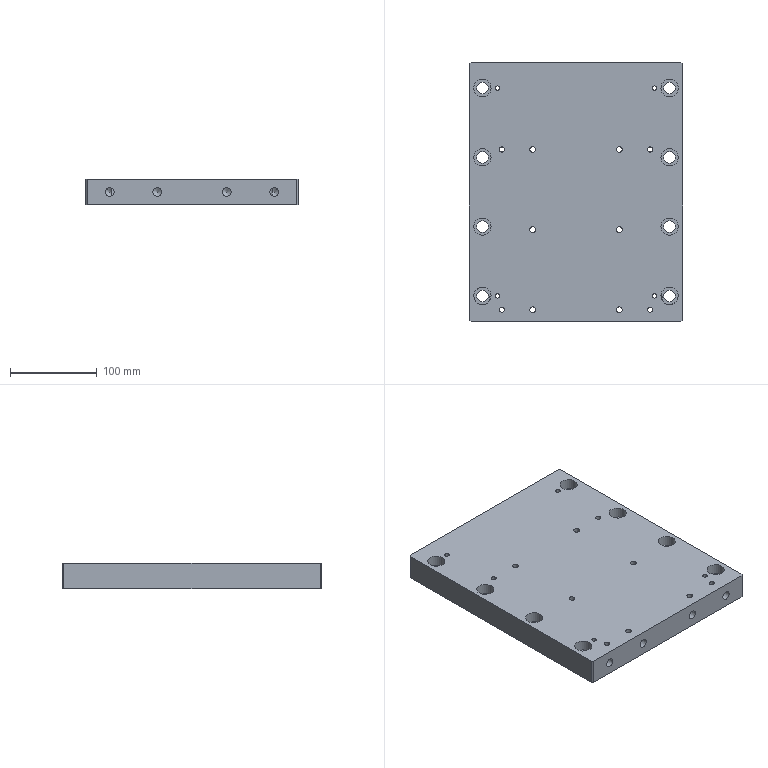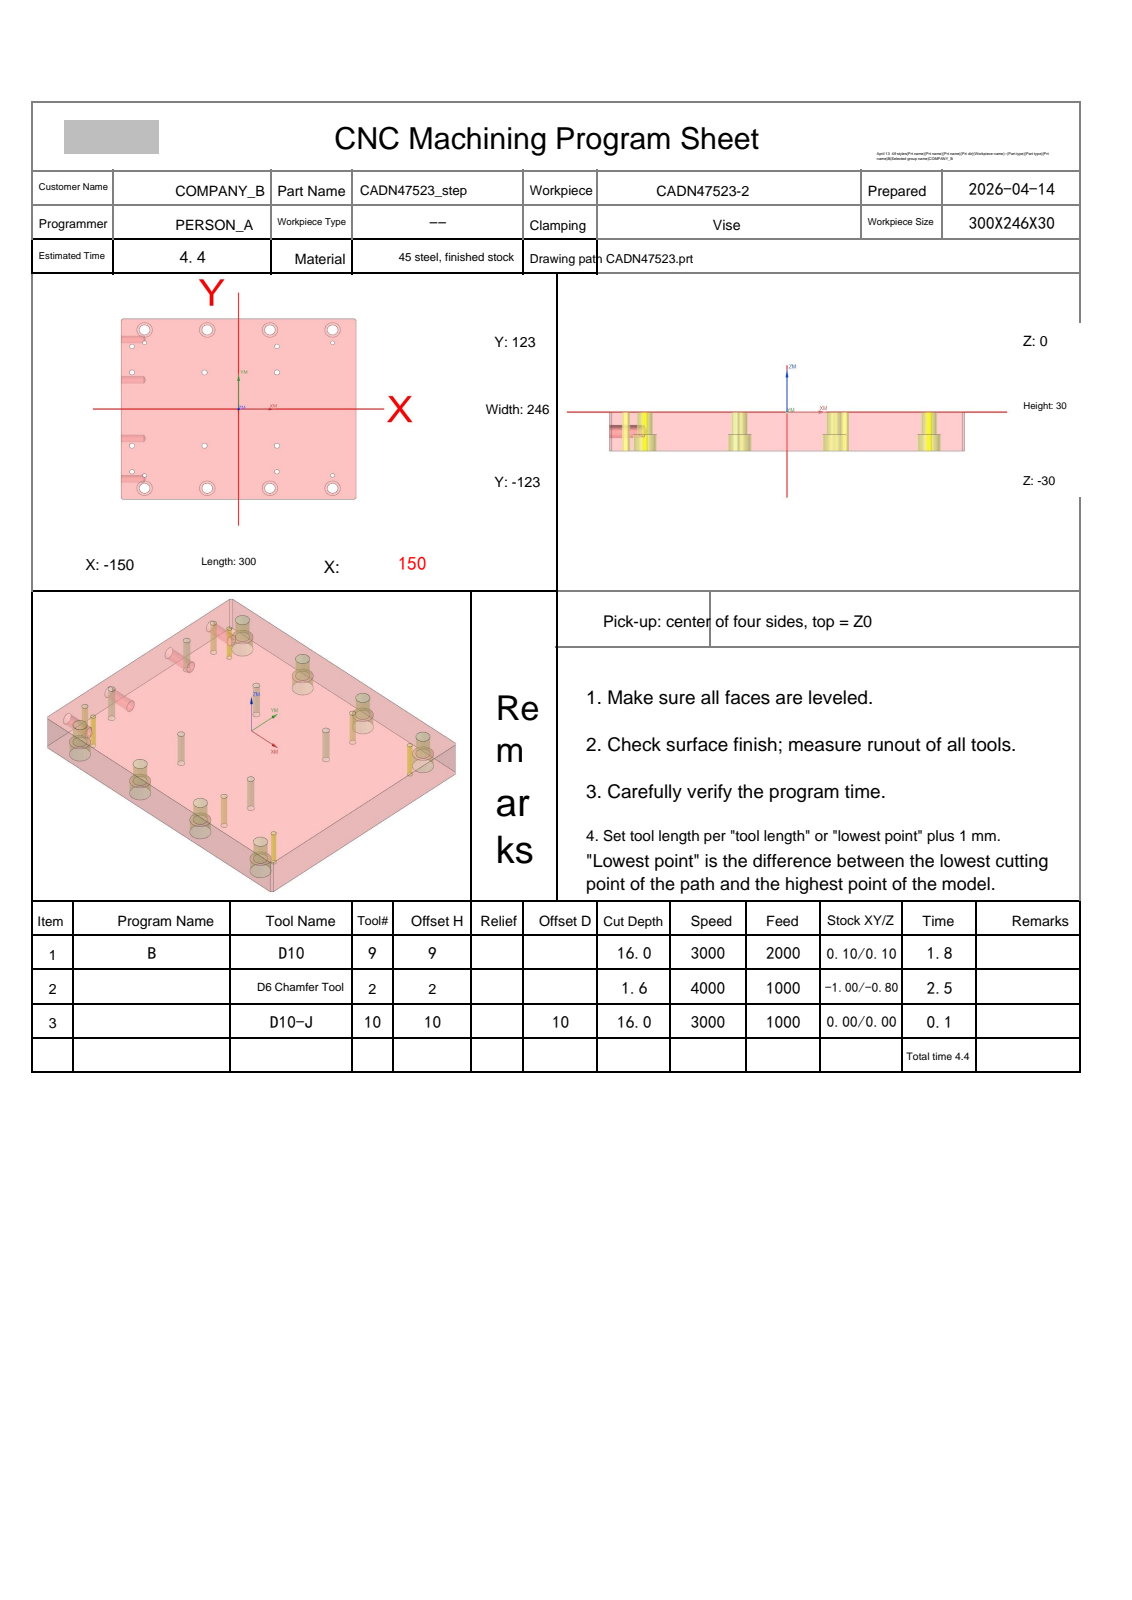NC program | NX | posted by the shop | part box 246 x 300 x 30 mm
Whole program:
%
O0001
(Machine time: 4.96 MIN)
(===Total Tool:3===)
(T9=D10     D=10.  R=0.   D-  H09 Z=-16.  )
(T2=D6 Chamfer Tool   D=6.   R=0.   D-  H02 Z=-1.6  )
(T10=D10-J  D=10.  R=0.   D10 H10 Z=-16.  )
G80 G90 G17 G49 G40
G91 G28 Z0
M01
N1 T09 M06
(D10  D=10. R=0. H=09 ce=0.10 di=0.10)
G00 G90 G54 X160.1 Y-118.112 M03 S3000
G43 H09 Z20.
M08
Z-.4
G01 X153.606 Y-124.606 F2000.
X151.606 Y-126.606
X145.112 Y-133.1
G00 Z-.8
G01 X151.606 Y-126.606
X153.606 Y-124.606
X160.1 Y-118.112
G00 Z-1.2
G01 X153.606 Y-124.606
X151.606 Y-126.606
X145.112 Y-133.1
G00 Z-1.6
G01 X151.606 Y-126.606
X153.606 Y-124.606
X160.1 Y-118.112
G00 Z-2.
G01 X153.606 Y-124.606
X151.606 Y-126.606
X145.112 Y-133.1
G00 Z-2.4
G01 X151.606 Y-126.606
X153.606 Y-124.606
X160.1 Y-118.112
G00 Z-2.8
G01 X153.606 Y-124.606
X151.606 Y-126.606
X145.112 Y-133.1
G00 Z-3.2
G01 X151.606 Y-126.606
X153.606 Y-124.606
X160.1 Y-118.112
G00 Z-3.6
G01 X153.606 Y-124.606
X151.606 Y-126.606
X145.112 Y-133.1
G00 Z-4.
G01 X151.606 Y-126.606
X153.606 Y-124.606
X160.1 Y-118.112
G00 Z-4.4
G01 X153.606 Y-124.606
X151.606 Y-126.606
X145.112 Y-133.1
G00 Z-4.8
G01 X151.606 Y-126.606
X153.606 Y-124.606
X160.1 Y-118.112
G00 Z-5.2
G01 X153.606 Y-124.606
X151.606 Y-126.606
X145.112 Y-133.1
G00 Z-5.6
G01 X151.606 Y-126.606
X153.606 Y-124.606
X160.1 Y-118.112
G00 Z-6.
G01 X153.606 Y-124.606
X151.606 Y-126.606
X145.112 Y-133.1
G00 Z-6.4
G01 X151.606 Y-126.606
X153.606 Y-124.606
X160.1 Y-118.112
G00 Z-6.8
G01 X153.606 Y-124.606
X151.606 Y-126.606
X145.112 Y-133.1
G00 Z-7.2
G01 X151.606 Y-126.606
X153.606 Y-124.606
X160.1 Y-118.112
G00 Z-7.6
G01 X153.606 Y-124.606
X151.606 Y-126.606
X145.112 Y-133.1
G00 Z-8.
G01 X151.606 Y-126.606
X153.606 Y-124.606
X160.1 Y-118.112
G00 Z-8.4
G01 X153.606 Y-124.606
X151.606 Y-126.606
X145.112 Y-133.1
G00 Z-8.8
G01 X151.606 Y-126.606
X153.606 Y-124.606
X160.1 Y-118.112
G00 Z-9.2
G01 X153.606 Y-124.606
X151.606 Y-126.606
X145.112 Y-133.1
G00 Z-9.6
G01 X151.606 Y-126.606
X153.606 Y-124.606
X160.1 Y-118.112
G00 Z-10.
G01 X153.606 Y-124.606
X151.606 Y-126.606
X145.112 Y-133.1
G00 Z-10.4
G01 X151.606 Y-126.606
X153.606 Y-124.606
X160.1 Y-118.112
G00 Z-10.8
G01 X153.606 Y-124.606
X151.606 Y-126.606
X145.112 Y-133.1
G00 Z-11.2
G01 X151.606 Y-126.606
X153.606 Y-124.606
X160.1 Y-118.112
G00 Z-11.6
G01 X153.606 Y-124.606
X151.606 Y-126.606
X145.112 Y-133.1
G00 Z-12.
G01 X151.606 Y-126.606
X153.606 Y-124.606
X160.1 Y-118.112
G00 Z-12.4
G01 X153.606 Y-124.606
X151.606 Y-126.606
X145.112 Y-133.1
G00 Z-12.8
G01 X151.606 Y-126.606
X153.606 Y-124.606
X160.1 Y-118.112
G00 Z-13.2
G01 X153.606 Y-124.606
X151.606 Y-126.606
X145.112 Y-133.1
G00 Z-13.6
G01 X151.606 Y-126.606
X153.606 Y-124.606
X160.1 Y-118.112
G00 Z-14.
G01 X153.606 Y-124.606
X151.606 Y-126.606
X145.112 Y-133.1
G00 Z-14.4
G01 X151.606 Y-126.606
X153.606 Y-124.606
X160.1 Y-118.112
G00 Z-14.8
G01 X153.606 Y-124.606
X151.606 Y-126.606
X145.112 Y-133.1
G00 Z-15.2
G01 X151.606 Y-126.606
X153.606 Y-124.606
X160.1 Y-118.112
G00 Z-15.6
G01 X153.606 Y-124.606
X151.606 Y-126.606
X145.112 Y-133.1
G00 Z-16.
G01 X151.606 Y-126.606
X153.606 Y-124.606
X160.1 Y-118.112
G00 Z20.
X145.112 Y133.1
Z-.4
G01 X151.606 Y126.606
X153.606 Y124.606
X160.1 Y118.112
G00 Z-.8
G01 X153.606 Y124.606
X151.606 Y126.606
X145.112 Y133.1
G00 Z-1.2
G01 X151.606 Y126.606
X153.606 Y124.606
X160.1 Y118.112
G00 Z-1.6
G01 X153.606 Y124.606
X151.606 Y126.606
X145.112 Y133.1
G00 Z-2.
G01 X151.606 Y126.606
X153.606 Y124.606
X160.1 Y118.112
G00 Z-2.4
G01 X153.606 Y124.606
X151.606 Y126.606
X145.112 Y133.1
G00 Z-2.8
G01 X151.606 Y126.606
X153.606 Y124.606
X160.1 Y118.112
G00 Z-3.2
G01 X153.606 Y124.606
X151.606 Y126.606
X145.112 Y133.1
G00 Z-3.6
G01 X151.606 Y126.606
X153.606 Y124.606
X160.1 Y118.112
G00 Z-4.
G01 X153.606 Y124.606
X151.606 Y126.606
X145.112 Y133.1
G00 Z-4.4
G01 X151.606 Y126.606
X153.606 Y124.606
X160.1 Y118.112
G00 Z-4.8
G01 X153.606 Y124.606
X151.606 Y126.606
X145.112 Y133.1
G00 Z-5.2
G01 X151.606 Y126.606
X153.606 Y124.606
X160.1 Y118.112
G00 Z-5.6
G01 X153.606 Y124.606
X151.606 Y126.606
X145.112 Y133.1
G00 Z-6.
G01 X151.606 Y126.606
X153.606 Y124.606
X160.1 Y118.112
G00 Z-6.4
G01 X153.606 Y124.606
X151.606 Y126.606
X145.112 Y133.1
G00 Z-6.8
G01 X151.606 Y126.606
X153.606 Y124.606
X160.1 Y118.112
G00 Z-7.2
G01 X153.606 Y124.606
X151.606 Y126.606
X145.112 Y133.1
G00 Z-7.6
G01 X151.606 Y126.606
X153.606 Y124.606
X160.1 Y118.112
G00 Z-8.
G01 X153.606 Y124.606
X151.606 Y126.606
X145.112 Y133.1
G00 Z-8.4
G01 X151.606 Y126.606
X153.606 Y124.606
X160.1 Y118.112
G00 Z-8.8
G01 X153.606 Y124.606
X151.606 Y126.606
X145.112 Y133.1
G00 Z-9.2
G01 X151.606 Y126.606
X153.606 Y124.606
X160.1 Y118.112
G00 Z-9.6
G01 X153.606 Y124.606
X151.606 Y126.606
X145.112 Y133.1
G00 Z-10.
G01 X151.606 Y126.606
X153.606 Y124.606
X160.1 Y118.112
G00 Z-10.4
G01 X153.606 Y124.606
X151.606 Y126.606
X145.112 Y133.1
G00 Z-10.8
G01 X151.606 Y126.606
X153.606 Y124.606
X160.1 Y118.112
G00 Z-11.2
G01 X153.606 Y124.606
X151.606 Y126.606
X145.112 Y133.1
G00 Z-11.6
G01 X151.606 Y126.606
X153.606 Y124.606
X160.1 Y118.112
G00 Z-12.
G01 X153.606 Y124.606
X151.606 Y126.606
X145.112 Y133.1
G00 Z-12.4
G01 X151.606 Y126.606
X153.606 Y124.606
X160.1 Y118.112
G00 Z-12.8
G01 X153.606 Y124.606
X151.606 Y126.606
X145.112 Y133.1
G00 Z-13.2
G01 X151.606 Y126.606
X153.606 Y124.606
X160.1 Y118.112
G00 Z-13.6
G01 X153.606 Y124.606
X151.606 Y126.606
X145.112 Y133.1
G00 Z-14.
G01 X151.606 Y126.606
X153.606 Y124.606
X160.1 Y118.112
G00 Z-14.4
G01 X153.606 Y124.606
X151.606 Y126.606
X145.112 Y133.1
G00 Z-14.8
G01 X151.606 Y126.606
X153.606 Y124.606
X160.1 Y118.112
G00 Z-15.2
G01 X153.606 Y124.606
X151.606 Y126.606
X145.112 Y133.1
G00 Z-15.6
G01 X151.606 Y126.606
X153.606 Y124.606
X160.1 Y118.112
G00 Z-16.
G01 X153.606 Y124.606
X151.606 Y126.606
X145.112 Y133.1
G00 Z20.
X-160.1 Y118.112
Z-.4
G01 X-153.606 Y124.606
X-151.606 Y126.606
X-145.112 Y133.1
G00 Z-.8
G01 X-151.606 Y126.606
X-153.606 Y124.606
X-160.1 Y118.112
G00 Z-1.2
G01 X-153.606 Y124.606
X-151.606 Y126.606
X-145.112 Y133.1
G00 Z-1.6
G01 X-151.606 Y126.606
X-153.606 Y124.606
X-160.1 Y118.112
G00 Z-2.
G01 X-153.606 Y124.606
X-151.606 Y126.606
X-145.112 Y133.1
G00 Z-2.4
G01 X-151.606 Y126.606
X-153.606 Y124.606
X-160.1 Y118.112
G00 Z-2.8
G01 X-153.606 Y124.606
X-151.606 Y126.606
X-145.112 Y133.1
G00 Z-3.2
G01 X-151.606 Y126.606
X-153.606 Y124.606
X-160.1 Y118.112
G00 Z-3.6
G01 X-153.606 Y124.606
X-151.606 Y126.606
X-145.112 Y133.1
G00 Z-4.
G01 X-151.606 Y126.606
X-153.606 Y124.606
X-160.1 Y118.112
G00 Z-4.4
G01 X-153.606 Y124.606
X-151.606 Y126.606
X-145.112 Y133.1
G00 Z-4.8
G01 X-151.606 Y126.606
X-153.606 Y124.606
X-160.1 Y118.112
G00 Z-5.2
G01 X-153.606 Y124.606
X-151.606 Y126.606
X-145.112 Y133.1
G00 Z-5.6
G01 X-151.606 Y126.606
X-153.606 Y124.606
X-160.1 Y118.112
G00 Z-6.
G01 X-153.606 Y124.606
X-151.606 Y126.606
X-145.112 Y133.1
G00 Z-6.4
G01 X-151.606 Y126.606
X-153.606 Y124.606
X-160.1 Y118.112
G00 Z-6.8
G01 X-153.606 Y124.606
X-151.606 Y126.606
X-145.112 Y133.1
G00 Z-7.2
G01 X-151.606 Y126.606
X-153.606 Y124.606
X-160.1 Y118.112
G00 Z-7.6
G01 X-153.606 Y124.606
X-151.606 Y126.606
X-145.112 Y133.1
G00 Z-8.
G01 X-151.606 Y126.606
X-153.606 Y124.606
X-160.1 Y118.112
G00 Z-8.4
G01 X-153.606 Y124.606
X-151.606 Y126.606
X-145.112 Y133.1
G00 Z-8.8
G01 X-151.606 Y126.606
X-153.606 Y124.606
X-160.1 Y118.112
G00 Z-9.2
G01 X-153.606 Y124.606
X-151.606 Y126.606
X-145.112 Y133.1
G00 Z-9.6
G01 X-151.606 Y126.606
X-153.606 Y124.606
X-160.1 Y118.112
G00 Z-10.
G01 X-153.606 Y124.606
X-151.606 Y126.606
X-145.112 Y133.1
G00 Z-10.4
G01 X-151.606 Y126.606
X-153.606 Y124.606
X-160.1 Y118.112
G00 Z-10.8
G01 X-153.606 Y124.606
X-151.606 Y126.606
X-145.112 Y133.1
G00 Z-11.2
G01 X-151.606 Y126.606
X-153.606 Y124.606
X-160.1 Y118.112
G00 Z-11.6
G01 X-153.606 Y124.606
X-151.606 Y126.606
X-145.112 Y133.1
G00 Z-12.
G01 X-151.606 Y126.606
X-153.606 Y124.606
X-160.1 Y118.112
G00 Z-12.4
G01 X-153.606 Y124.606
X-151.606 Y126.606
X-145.112 Y133.1
G00 Z-12.8
G01 X-151.606 Y126.606
X-153.606 Y124.606
X-160.1 Y118.112
G00 Z-13.2
G01 X-153.606 Y124.606
X-151.606 Y126.606
X-145.112 Y133.1
G00 Z-13.6
G01 X-151.606 Y126.606
X-153.606 Y124.606
X-160.1 Y118.112
G00 Z-14.
G01 X-153.606 Y124.606
X-151.606 Y126.606
X-145.112 Y133.1
G00 Z-14.4
G01 X-151.606 Y126.606
X-153.606 Y124.606
X-160.1 Y118.112
G00 Z-14.8
G01 X-153.606 Y124.606
X-151.606 Y126.606
X-145.112 Y133.1
G00 Z-15.2
G01 X-151.606 Y126.606
X-153.606 Y124.606
X-160.1 Y118.112
G00 Z-15.6
G01 X-153.606 Y124.606
X-151.606 Y126.606
X-145.112 Y133.1
G00 Z-16.
G01 X-151.606 Y126.606
X-153.606 Y124.606
X-160.1 Y118.112
G00 Z20.
X-145.112 Y-133.1
Z-.4
G01 X-151.606 Y-126.606
X-153.606 Y-124.606
X-160.1 Y-118.112
G00 Z-.8
G01 X-153.606 Y-124.606
X-151.606 Y-126.606
X-145.112 Y-133.1
G00 Z-1.2
G01 X-151.606 Y-126.606
X-153.606 Y-124.606
X-160.1 Y-118.112
G00 Z-1.6
G01 X-153.606 Y-124.606
X-151.606 Y-126.606
X-145.112 Y-133.1
G00 Z-2.
G01 X-151.606 Y-126.606
X-153.606 Y-124.606
X-160.1 Y-118.112
G00 Z-2.4
G01 X-153.606 Y-124.606
X-151.606 Y-126.606
X-145.112 Y-133.1
G00 Z-2.8
G01 X-151.606 Y-126.606
X-153.606 Y-124.606
X-160.1 Y-118.112
G00 Z-3.2
G01 X-153.606 Y-124.606
X-151.606 Y-126.606
X-145.112 Y-133.1
G00 Z-3.6
G01 X-151.606 Y-126.606
X-153.606 Y-124.606
X-160.1 Y-118.112
G00 Z-4.
G01 X-153.606 Y-124.606
X-151.606 Y-126.606
X-145.112 Y-133.1
G00 Z-4.4
G01 X-151.606 Y-126.606
X-153.606 Y-124.606
X-160.1 Y-118.112
G00 Z-4.8
G01 X-153.606 Y-124.606
X-151.606 Y-126.606
X-145.112 Y-133.1
G00 Z-5.2
G01 X-151.606 Y-126.606
X-153.606 Y-124.606
X-160.1 Y-118.112
G00 Z-5.6
G01 X-153.606 Y-124.606
X-151.606 Y-126.606
X-145.112 Y-133.1
G00 Z-6.
G01 X-151.606 Y-126.606
X-153.606 Y-124.606
X-160.1 Y-118.112
G00 Z-6.4
G01 X-153.606 Y-124.606
X-151.606 Y-126.606
X-145.112 Y-133.1
G00 Z-6.8
G01 X-151.606 Y-126.606
X-153.606 Y-124.606
X-160.1 Y-118.112
G00 Z-7.2
G01 X-153.606 Y-124.606
X-151.606 Y-126.606
X-145.112 Y-133.1
G00 Z-7.6
G01 X-151.606 Y-126.606
X-153.606 Y-124.606
X-160.1 Y-118.112
G00 Z-8.
G01 X-153.606 Y-124.606
X-151.606 Y-126.606
X-145.112 Y-133.1
G00 Z-8.4
G01 X-151.606 Y-126.606
X-153.606 Y-124.606
X-160.1 Y-118.112
G00 Z-8.8
G01 X-153.606 Y-124.606
X-151.606 Y-126.606
X-145.112 Y-133.1
G00 Z-9.2
G01 X-151.606 Y-126.606
X-153.606 Y-124.606
X-160.1 Y-118.112
G00 Z-9.6
G01 X-153.606 Y-124.606
X-151.606 Y-126.606
X-145.112 Y-133.1
G00 Z-10.
G01 X-151.606 Y-126.606
X-153.606 Y-124.606
X-160.1 Y-118.112
G00 Z-10.4
G01 X-153.606 Y-124.606
X-151.606 Y-126.606
X-145.112 Y-133.1
G00 Z-10.8
G01 X-151.606 Y-126.606
X-153.606 Y-124.606
X-160.1 Y-118.112
G00 Z-11.2
G01 X-153.606 Y-124.606
X-151.606 Y-126.606
X-145.112 Y-133.1
G00 Z-11.6
G01 X-151.606 Y-126.606
X-153.606 Y-124.606
X-160.1 Y-118.112
G00 Z-12.
G01 X-153.606 Y-124.606
X-151.606 Y-126.606
X-145.112 Y-133.1
G00 Z-12.4
G01 X-151.606 Y-126.606
X-153.606 Y-124.606
X-160.1 Y-118.112
G00 Z-12.8
G01 X-153.606 Y-124.606
X-151.606 Y-126.606
X-145.112 Y-133.1
G00 Z-13.2
G01 X-151.606 Y-126.606
X-153.606 Y-124.606
X-160.1 Y-118.112
G00 Z-13.6
G01 X-153.606 Y-124.606
X-151.606 Y-126.606
X-145.112 Y-133.1
G00 Z-14.
G01 X-151.606 Y-126.606
X-153.606 Y-124.606
X-160.1 Y-118.112
G00 Z-14.4
G01 X-153.606 Y-124.606
X-151.606 Y-126.606
X-145.112 Y-133.1
G00 Z-14.8
G01 X-151.606 Y-126.606
X-153.606 Y-124.606
X-160.1 Y-118.112
G00 Z-15.2
G01 X-153.606 Y-124.606
X-151.606 Y-126.606
X-145.112 Y-133.1
G00 Z-15.6
G01 X-151.606 Y-126.606
X-153.606 Y-124.606
X-160.1 Y-118.112
G00 Z-16.
G01 X-153.606 Y-124.606
X-151.606 Y-126.606
X-145.112 Y-133.1
G00 Z20.
G91 G28 Z0.0
M05
M09
G91 G28 Z0.0
M01
N2 T02 M06
(D6 Chamfer Tool  D=6. R=0. H=02 ce=-0.30 di=-0.80)
G00 G90 G54 X-119.81 Y90.563 M03 S4000
G43 H02 Z20.
M08
Z-1.1
G01 Z-1.6 F600.
X-119.776 Y90.574
G03 X-119.747 Y90.867 I-1.471 J.293
X-120. Y91.7 I-1.5 J0.0
X-121.2 Y90.5 I0.0 J-1.2
X-120. Y89.3 I1.2 J0.0
X-118.8 Y90.5 I0.0 J1.2
X-120. Y91.7 I-1.2 J0.0
X-120.253 Y90.867 I1.247 J-.833
X-120.224 Y90.574 I1.5 J0.0
G01 X-120.19 Y90.563
Z-1.1
G00 Z20.
X-119.81 Y-90.437
Z-1.1
G01 Z-1.6
X-119.776 Y-90.426
G03 X-119.747 Y-90.133 I-1.471 J.293
X-120. Y-89.3 I-1.5 J0.0
X-121.2 Y-90.5 I0.0 J-1.2
X-120. Y-91.7 I1.2 J0.0
X-118.8 Y-90.5 I0.0 J1.2
X-120. Y-89.3 I-1.2 J0.0
X-120.253 Y-90.133 I1.247 J-.833
X-120.224 Y-90.426 I1.5 J0.0
G01 X-120.19 Y-90.437
Z-1.1
G00 Z20.
X120.19
Z-1.1
G01 Z-1.6
X120.224 Y-90.426
G03 X120.253 Y-90.133 I-1.471 J.293
X120. Y-89.3 I-1.5 J0.0
X118.8 Y-90.5 I0.0 J-1.2
X120. Y-91.7 I1.2 J0.0
X121.2 Y-90.5 I0.0 J1.2
X120. Y-89.3 I-1.2 J0.0
X119.747 Y-90.133 I1.247 J-.833
X119.776 Y-90.426 I1.5 J0.0
G01 X119.81 Y-90.437
Z-1.1
G00 Z20.
X120.19 Y90.563
Z-1.1
G01 Z-1.6
X120.224 Y90.574
G03 X120.253 Y90.867 I-1.471 J.293
X120. Y91.7 I-1.5 J0.0
X118.8 Y90.5 I0.0 J-1.2
X120. Y89.3 I1.2 J0.0
X121.2 Y90.5 I0.0 J1.2
X120. Y91.7 I-1.2 J0.0
X119.747 Y90.867 I1.247 J-.833
X119.776 Y90.574 I1.5 J0.0
G01 X119.81 Y90.563
Z-1.1
G00 Z20.
G00 G90 X48.306 Y-85.593 M03 S4000
Z20.
Z-1.1
G01 Z-1.6 F600.
X47.5 Y-85.7
G03 X49. Y-87.2 I1.5 J0.0
X50.7 Y-85.5 I0.0 J1.7
X49. Y-83.8 I-1.7 J0.0
X47.3 Y-85.5 I0.0 J-1.7
X49. Y-87.2 I1.7 J0.0
X50.5 Y-85.7 I0.0 J1.5
G01 X49.694 Y-85.593
Z-1.1
G00 Z20.
X48.306 Y85.407
Z-1.1
G01 Z-1.6
X47.5 Y85.3
G03 X49. Y83.8 I1.5 J0.0
X50.7 Y85.5 I0.0 J1.7
X49. Y87.2 I-1.7 J0.0
X47.3 Y85.5 I0.0 J-1.7
X49. Y83.8 I1.7 J0.0
X50.5 Y85.3 I0.0 J1.5
G01 X49.694 Y85.407
Z-1.1
G00 Z20.
X-136.694
Z-1.1
G01 Z-1.6
X-137.5 Y85.3
G03 X-136. Y83.8 I1.5 J0.0
X-134.3 Y85.5 I0.0 J1.7
X-136. Y87.2 I-1.7 J0.0
X-137.7 Y85.5 I0.0 J-1.7
X-136. Y83.8 I1.7 J0.0
X-134.5 Y85.3 I0.0 J1.5
G01 X-135.306 Y85.407
Z-1.1
G00 Z20.
X-136.694 Y-85.593
Z-1.1
G01 Z-1.6
X-137.5 Y-85.7
G03 X-136. Y-87.2 I1.5 J0.0
X-134.3 Y-85.5 I0.0 J1.7
X-136. Y-83.8 I-1.7 J0.0
X-137.7 Y-85.5 I0.0 J-1.7
X-136. Y-87.2 I1.7 J0.0
X-134.5 Y-85.7 I0.0 J1.5
G01 X-135.306 Y-85.593
Z-1.1
G00 Z20.
G00 G90 X-134.5 Y50.995 M03 S4000
Z20.
Z-1.1
G01 Z-1.6 F300.
Y51.3
G03 X-136. Y52.8 I-1.5 J0.0
X-138.8 Y50. I0.0 J-2.8
X-136. Y47.2 I2.8 J0.0
X-133.2 Y50. I0.0 J2.8
X-136. Y52.8 I-2.8 J0.0
X-137.5 Y51.3 I0.0 J-1.5
G01 Y50.995
Z-1.1
G00 Z20.
X-42.
Z-1.1
G01 Z-1.6
Y51.3
G03 X-43.5 Y52.8 I-1.5 J0.0
X-46.3 Y50. I0.0 J-2.8
X-43.5 Y47.2 I2.8 J0.0
X-40.7 Y50. I0.0 J2.8
X-43.5 Y52.8 I-2.8 J0.0
X-45. Y51.3 I0.0 J-1.5
G01 Y50.995
Z-1.1
G00 Z20.
X50.5
Z-1.1
G01 Z-1.6
Y51.3
G03 X49. Y52.8 I-1.5 J0.0
X46.2 Y50. I0.0 J-2.8
X49. Y47.2 I2.8 J0.0
X51.8 Y50. I0.0 J2.8
X49. Y52.8 I-2.8 J0.0
X47.5 Y51.3 I0.0 J-1.5
G01 Y50.995
Z-1.1
G00 Z20.
X50.5 Y-49.005
Z-1.1
G01 Z-1.6
Y-48.7
G03 X49. Y-47.2 I-1.5 J0.0
X46.2 Y-50. I0.0 J-2.8
X49. Y-52.8 I2.8 J0.0
X51.8 Y-50. I0.0 J2.8
X49. Y-47.2 I-2.8 J0.0
X47.5 Y-48.7 I0.0 J-1.5
G01 Y-49.005
Z-1.1
G00 Z20.
X-42.
Z-1.1
G01 Z-1.6
Y-48.7
G03 X-43.5 Y-47.2 I-1.5 J0.0
X-46.3 Y-50. I0.0 J-2.8
X-43.5 Y-52.8 I2.8 J0.0
X-40.7 Y-50. I0.0 J2.8
X-43.5 Y-47.2 I-2.8 J0.0
X-45. Y-48.7 I0.0 J-1.5
G01 Y-49.005
Z-1.1
G00 Z20.
X-134.5
Z-1.1
G01 Z-1.6
Y-48.7
G03 X-136. Y-47.2 I-1.5 J0.0
X-138.8 Y-50. I0.0 J-2.8
X-136. Y-52.8 I2.8 J0.0
X-133.2 Y-50. I0.0 J2.8
X-136. Y-47.2 I-2.8 J0.0
X-137.5 Y-48.7 I0.0 J-1.5
G01 Y-49.005
Z-1.1
G00 Z20.
G00 G90 X125.578 Y-109.392 M03 S4000
Z20.
Z2.5
G01 X125.606 Y-109.292 Z2.462 F1000.
X125.698 Y-108.793 Z2.278
X125.746 Y-108.288 Z2.093
X125.749 Y-107.78 Z1.908
X125.707 Y-107.274 Z1.723
X125.621 Y-106.774 Z1.539
X125.491 Y-106.284 Z1.354
X125.318 Y-105.806 Z1.169
X125.104 Y-105.346 Z.984
X124.851 Y-104.907 Z.8
X124.559 Y-104.491 Z.615
X124.232 Y-104.103 Z.43
X123.872 Y-103.745 Z.245
X123.482 Y-103.42 Z.061
X123.065 Y-103.131 Z-.124
X122.624 Y-102.88 Z-.309
X122.162 Y-102.669 Z-.493
X121.684 Y-102.499 Z-.678
X121.193 Y-102.372 Z-.863
X120.692 Y-102.289 Z-1.048
X120.186 Y-102.25 Z-1.232
X120. Z-1.3
G03 X114.25 Y-108. I0.0 J-5.75
X120. Y-113.75 I5.75 J0.0
X125.75 Y-108. I0.0 J5.75
X120. Y-102.25 I-5.75 J0.0
X119.501 Y-102.272 I0.0 J-5.75
G01 Z1.2
G00 Z20.
X45.578 Y-109.392
Z2.5
G01 X45.606 Y-109.292 Z2.462
X45.698 Y-108.793 Z2.278
X45.746 Y-108.288 Z2.093
X45.749 Y-107.78 Z1.908
X45.707 Y-107.274 Z1.723
X45.621 Y-106.774 Z1.539
X45.491 Y-106.284 Z1.354
X45.318 Y-105.806 Z1.169
X45.104 Y-105.346 Z.984
X44.851 Y-104.907 Z.8
X44.559 Y-104.491 Z.615
X44.232 Y-104.103 Z.43
X43.872 Y-103.745 Z.245
X43.482 Y-103.42 Z.061
X43.065 Y-103.131 Z-.124
X42.624 Y-102.88 Z-.309
X42.162 Y-102.669 Z-.493
X41.684 Y-102.499 Z-.678
X41.193 Y-102.372 Z-.863
X40.692 Y-102.289 Z-1.048
X40.186 Y-102.25 Z-1.232
X40. Z-1.3
G03 X34.25 Y-108. I0.0 J-5.75
X40. Y-113.75 I5.75 J0.0
X45.75 Y-108. I0.0 J5.75
X40. Y-102.25 I-5.75 J0.0
X39.501 Y-102.272 I0.0 J-5.75
G01 Z1.2
G00 Z20.
X-34.422 Y-109.392
Z2.5
G01 X-34.394 Y-109.292 Z2.462
X-34.302 Y-108.793 Z2.278
X-34.254 Y-108.288 Z2.093
X-34.251 Y-107.78 Z1.908
X-34.293 Y-107.274 Z1.723
X-34.379 Y-106.774 Z1.539
X-34.509 Y-106.284 Z1.354
X-34.682 Y-105.806 Z1.169
X-34.896 Y-105.346 Z.984
X-35.149 Y-104.907 Z.8
X-35.441 Y-104.491 Z.615
X-35.768 Y-104.103 Z.43
X-36.128 Y-103.745 Z.245
X-36.518 Y-103.42 Z.061
X-36.935 Y-103.131 Z-.124
X-37.376 Y-102.88 Z-.309
X-37.838 Y-102.669 Z-.493
X-38.316 Y-102.499 Z-.678
X-38.807 Y-102.372 Z-.863
X-39.308 Y-102.289 Z-1.048
X-39.814 Y-102.25 Z-1.232
X-40. Z-1.3
G03 X-45.75 Y-108. I0.0 J-5.75
X-40. Y-113.75 I5.75 J0.0
X-34.25 Y-108. I0.0 J5.75
X-40. Y-102.25 I-5.75 J0.0
X-40.499 Y-102.272 I0.0 J-5.75
G01 Z1.2
G00 Z20.
X-114.422 Y-109.392
Z2.5
G01 X-114.394 Y-109.292 Z2.462
X-114.302 Y-108.793 Z2.278
X-114.254 Y-108.288 Z2.093
X-114.251 Y-107.78 Z1.908
X-114.293 Y-107.274 Z1.723
X-114.379 Y-106.774 Z1.539
X-114.509 Y-106.284 Z1.354
X-114.682 Y-105.806 Z1.169
X-114.896 Y-105.346 Z.984
X-115.149 Y-104.907 Z.8
X-115.441 Y-104.491 Z.615
X-115.768 Y-104.103 Z.43
X-116.128 Y-103.745 Z.245
X-116.518 Y-103.42 Z.061
X-116.935 Y-103.131 Z-.124
X-117.376 Y-102.88 Z-.309
X-117.838 Y-102.669 Z-.493
X-118.316 Y-102.499 Z-.678
X-118.807 Y-102.372 Z-.863
X-119.308 Y-102.289 Z-1.048
X-119.814 Y-102.25 Z-1.232
X-120. Z-1.3
G03 X-125.75 Y-108. I0.0 J-5.75
X-120. Y-113.75 I5.75 J0.0
X-114.25 Y-108. I0.0 J5.75
X-120. Y-102.25 I-5.75 J0.0
X-120.499 Y-102.272 I0.0 J-5.75
G01 Z1.2
G00 Z20.
X-151. Y111.458
Z2.5
G01 Y120.876 Z-.928
Y120.964 Z-.96
X-150.969 Y121.173 Z-1.037
X-150.904 Y121.374 Z-1.114
X-150.807 Y121.562 Z-1.191
X-150.682 Y121.732 Z-1.268
X-150.619 Y121.795 Z-1.3
X-148.795 Y123.619
G02 X-147.876 Y124. I.919 J-.919
G01 X147.876
G02 X148.795 Y123.619 I0.0 J-1.3
G01 X150.619 Y121.795
G02 X151. Y120.876 I-.919 J-.919
G01 Y-120.876
G02 X150.619 Y-121.795 I-1.3 J0.0
G01 X148.795 Y-123.619
G02 X147.876 Y-124. I-.919 J.919
G01 X-147.876
G02 X-148.795 Y-123.619 I0.0 J1.3
G01 X-150.619 Y-121.795
G02 X-151. Y-120.876 I.919 J.919
G01 Y120.876
G02 X-150.619 Y121.795 I1.3 J0.0
G01 X-150.266 Y122.149
Z1.2
G00 Z20.
X-114.422 Y106.608
Z2.5
G01 X-114.394 Y106.708 Z2.462
X-114.302 Y107.207 Z2.278
X-114.254 Y107.712 Z2.093
X-114.251 Y108.22 Z1.908
X-114.293 Y108.726 Z1.723
X-114.379 Y109.226 Z1.539
X-114.509 Y109.716 Z1.354
X-114.682 Y110.194 Z1.169
X-114.896 Y110.654 Z.984
X-115.149 Y111.093 Z.8
X-115.441 Y111.509 Z.615
X-115.768 Y111.897 Z.43
X-116.128 Y112.255 Z.245
X-116.518 Y112.58 Z.061
X-116.935 Y112.869 Z-.124
X-117.376 Y113.12 Z-.309
X-117.838 Y113.331 Z-.493
X-118.316 Y113.501 Z-.678
X-118.807 Y113.628 Z-.863
X-119.308 Y113.711 Z-1.048
X-119.814 Y113.75 Z-1.232
X-120. Z-1.3
G03 X-125.75 Y108. I0.0 J-5.75
X-120. Y102.25 I5.75 J0.0
X-114.25 Y108. I0.0 J5.75
X-120. Y113.75 I-5.75 J0.0
X-120.499 Y113.728 I0.0 J-5.75
G01 Z1.2
G00 Z20.
X-34.422 Y106.608
Z2.5
G01 X-34.394 Y106.708 Z2.462
X-34.302 Y107.207 Z2.278
X-34.254 Y107.712 Z2.093
X-34.251 Y108.22 Z1.908
X-34.293 Y108.726 Z1.723
X-34.379 Y109.226 Z1.539
X-34.509 Y109.716 Z1.354
X-34.682 Y110.194 Z1.169
X-34.896 Y110.654 Z.984
X-35.149 Y111.093 Z.8
X-35.441 Y111.509 Z.615
X-35.768 Y111.897 Z.43
X-36.128 Y112.255 Z.245
X-36.518 Y112.58 Z.061
X-36.935 Y112.869 Z-.124
X-37.376 Y113.12 Z-.309
X-37.838 Y113.331 Z-.493
X-38.316 Y113.501 Z-.678
X-38.807 Y113.628 Z-.863
X-39.308 Y113.711 Z-1.048
X-39.814 Y113.75 Z-1.232
X-40. Z-1.3
G03 X-45.75 Y108. I0.0 J-5.75
X-40. Y102.25 I5.75 J0.0
X-34.25 Y108. I0.0 J5.75
X-40. Y113.75 I-5.75 J0.0
X-40.499 Y113.728 I0.0 J-5.75
G01 Z1.2
G00 Z20.
X45.578 Y106.608
Z2.5
G01 X45.606 Y106.708 Z2.462
X45.698 Y107.207 Z2.278
X45.746 Y107.712 Z2.093
X45.749 Y108.22 Z1.908
X45.707 Y108.726 Z1.723
X45.621 Y109.226 Z1.539
X45.491 Y109.716 Z1.354
X45.318 Y110.194 Z1.169
X45.104 Y110.654 Z.984
X44.851 Y111.093 Z.8
X44.559 Y111.509 Z.615
X44.232 Y111.897 Z.43
X43.872 Y112.255 Z.245
X43.482 Y112.58 Z.061
X43.065 Y112.869 Z-.124
X42.624 Y113.12 Z-.309
X42.162 Y113.331 Z-.493
X41.684 Y113.501 Z-.678
X41.193 Y113.628 Z-.863
X40.692 Y113.711 Z-1.048
X40.186 Y113.75 Z-1.232
X40. Z-1.3
G03 X34.25 Y108. I0.0 J-5.75
X40. Y102.25 I5.75 J0.0
X45.75 Y108. I0.0 J5.75
X40. Y113.75 I-5.75 J0.0
X39.501 Y113.728 I0.0 J-5.75
G01 Z1.2
G00 Z20.
X125.578 Y106.608
Z2.5
G01 X125.606 Y106.708 Z2.462
X125.698 Y107.207 Z2.278
X125.746 Y107.712 Z2.093
X125.749 Y108.22 Z1.908
X125.707 Y108.726 Z1.723
X125.621 Y109.226 Z1.539
X125.491 Y109.716 Z1.354
X125.318 Y110.194 Z1.169
X125.104 Y110.654 Z.984
X124.851 Y111.093 Z.8
X124.559 Y111.509 Z.615
X124.232 Y111.897 Z.43
X123.872 Y112.255 Z.245
X123.482 Y112.58 Z.061
X123.065 Y112.869 Z-.124
X122.624 Y113.12 Z-.309
X122.162 Y113.331 Z-.493
X121.684 Y113.501 Z-.678
X121.193 Y113.628 Z-.863
X120.692 Y113.711 Z-1.048
X120.186 Y113.75 Z-1.232
X120. Z-1.3
G03 X114.25 Y108. I0.0 J-5.75
X120. Y102.25 I5.75 J0.0
X125.75 Y108. I0.0 J5.75
X120. Y113.75 I-5.75 J0.0
X119.501 Y113.728 I0.0 J-5.75
G01 Z1.2
G00 Z20.
G91 G28 Z0.0
M05
M09
G91 G28 Z0.0
M01
N3 T10 M06
(D10-J  D=10. R=0. H=10 ce=0.00 di=0.00)
G00 G90 G54 X155.684 Y-124.544 M03 S3000
G43 H10 Z5.
M08
Z-15.
G01 Z-16. F1000.
G41 D10
X155.527 Y-124.42
G03 X154.596 Y-124.096 I-.931 J-1.176
X153.536 Y-124.536 I0.0 J-1.5
G01 X151.536 Y-126.536
G03 X151.096 Y-127.596 I1.061 J-1.061
X151.42 Y-128.527 I1.5 J0.0
G01 G40 X151.544 Y-128.684
Z-15.
G00 Z5.
Y128.684
Z-15.
G01 Z-16.
G41 D10
X151.42 Y128.527
G03 X151.096 Y127.596 I1.176 J-.931
X151.536 Y126.536 I1.5 J0.0
G01 X153.536 Y124.536
G03 X154.596 Y124.096 I1.061 J1.061
X155.527 Y124.42 I0.0 J1.5
G01 G40 X155.684 Y124.544
Z-15.
G00 Z5.
X-155.684
Z-15.
G01 Z-16.
G41 D10
X-155.527 Y124.42
G03 X-154.596 Y124.096 I.931 J1.176
X-153.536 Y124.536 I0.0 J1.5
G01 X-151.536 Y126.536
G03 X-151.096 Y127.596 I-1.061 J1.061
X-151.42 Y128.527 I-1.5 J0.0
G01 G40 X-151.544 Y128.684
Z-15.
G00 Z5.
Y-128.684
Z-15.
G01 Z-16.
G41 D10
X-151.42 Y-128.527
G03 X-151.096 Y-127.596 I-1.176 J.931
X-151.536 Y-126.536 I-1.5 J0.0
G01 X-153.536 Y-124.536
G03 X-154.596 Y-124.096 I-1.061 J-1.061
X-155.527 Y-124.42 I0.0 J-1.5
G01 G40 X-155.684 Y-124.544
Z-15.
G00 Z5.
M05
M09
G91 G28 Z0.0
G91 G28 Y0.0
M30
%